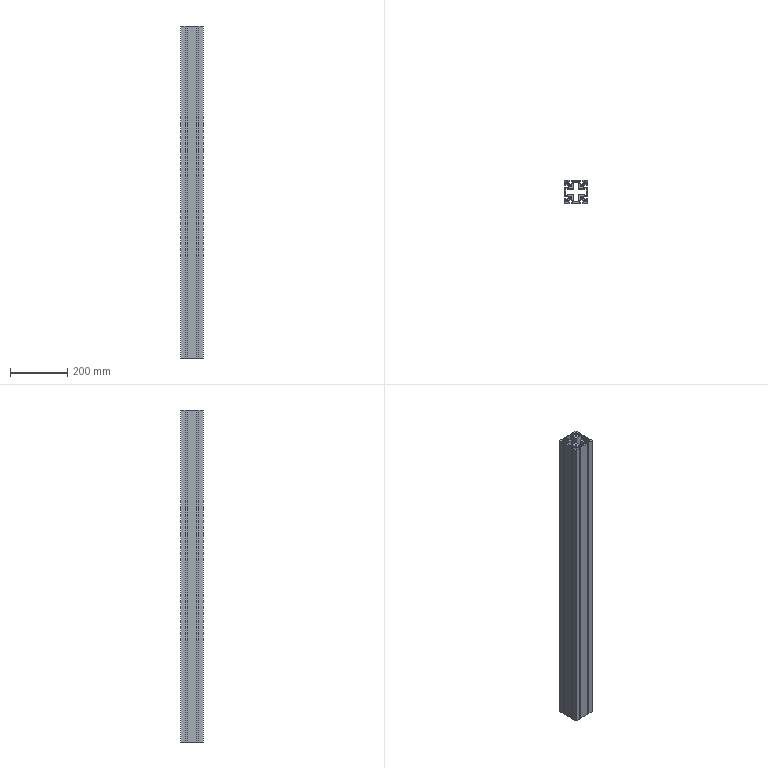Part | NX | features BREP 1 | 1 solid | 130 faces | box 80 x 80 x 1160 mm | volume 2854372 mm3 | plane 114 | cylinder 16 | commonest cylinder face diameters 6.8 x16